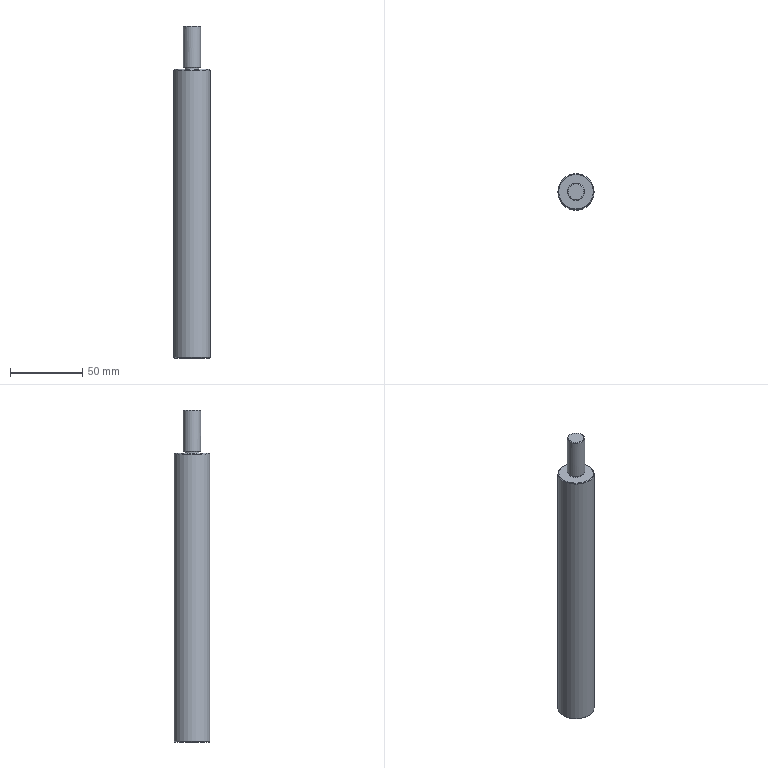Part | NX | features clamp shaft 2 | 1 solid | 13 faces | box 25 x 25 x 230 mm | volume 95439 mm3 | cone 5 | plane 4 | cylinder 4 | commonest cylinder face diameters 10 x1 12 x1 14 x1 25 x1
STEP:
#1=CARTESIAN_POINT('',(-5.5,0.,230.));
#2=VERTEX_POINT('',#1);
#3=CARTESIAN_POINT('',(0.,0.,230.));
#4=DIRECTION('',(0.,0.,-1.));
#5=DIRECTION('',(-1.,0.,0.));
#6=AXIS2_PLACEMENT_3D('',#3,#4,#5);
#7=CIRCLE('',#6,5.5);
#8=EDGE_CURVE('',#2,#2,#7,.T.);
#9=ORIENTED_EDGE('',*,*,#8,.F.);
#10=EDGE_LOOP('',(#9));
#11=FACE_BOUND('',#10,.T.);
#12=CARTESIAN_POINT('',(0.,0.,230.));
#13=DIRECTION('',(0.,0.,1.));
#14=DIRECTION('',(1.,0.,0.));
#15=AXIS2_PLACEMENT_3D('',#12,#13,#14);
#16=PLANE('',#15);
#17=ADVANCED_FACE('',(#11),#16,.T.);
#18=ORIENTED_EDGE('',*,*,#8,.T.);
#19=EDGE_LOOP('',(#18));
#20=FACE_BOUND('',#19,.T.);
#21=CARTESIAN_POINT('',(-6.,0.,229.5));
#22=VERTEX_POINT('',#21);
#23=CARTESIAN_POINT('',(0.,0.,229.5));
#24=DIRECTION('',(0.,0.,-1.));
#25=DIRECTION('',(-1.,0.,0.));
#26=AXIS2_PLACEMENT_3D('',#23,#24,#25);
#27=CIRCLE('',#26,6.);
#28=EDGE_CURVE('',#22,#22,#27,.T.);
#29=ORIENTED_EDGE('',*,*,#28,.F.);
#30=EDGE_LOOP('',(#29));
#31=FACE_BOUND('',#30,.T.);
#32=CARTESIAN_POINT('',(0.,0.,229.5));
#33=DIRECTION('',(0.,0.,-1.));
#34=DIRECTION('',(-1.,0.,0.));
#35=AXIS2_PLACEMENT_3D('',#32,#33,#34);
#36=CONICAL_SURFACE('',#35,6.,0.7854);
#37=ADVANCED_FACE('',(#20,#31),#36,.T.);
#38=ORIENTED_EDGE('',*,*,#28,.T.);
#39=EDGE_LOOP('',(#38));
#40=FACE_BOUND('',#39,.T.);
#41=CARTESIAN_POINT('',(6.,0.,201.5));
#42=VERTEX_POINT('',#41);
#43=CARTESIAN_POINT('',(0.,0.,201.5));
#44=DIRECTION('',(0.,0.,1.));
#45=DIRECTION('',(1.,0.,0.));
#46=AXIS2_PLACEMENT_3D('',#43,#44,#45);
#47=CIRCLE('',#46,6.);
#48=EDGE_CURVE('',#42,#42,#47,.F.);
#49=ORIENTED_EDGE('',*,*,#48,.F.);
#50=EDGE_LOOP('',(#49));
#51=FACE_BOUND('',#50,.T.);
#52=CARTESIAN_POINT('',(0.,0.,230.));
#53=DIRECTION('',(0.,0.,-1.));
#54=DIRECTION('',(-1.,0.,0.));
#55=AXIS2_PLACEMENT_3D('',#52,#53,#54);
#56=CYLINDRICAL_SURFACE('',#55,6.);
#57=ADVANCED_FACE('',(#40,#51),#56,.T.);
#58=CARTESIAN_POINT('',(0.,-5.5,201.));
#59=VERTEX_POINT('',#58);
#60=CARTESIAN_POINT('',(0.,0.,201.));
#61=DIRECTION('',(0.,0.,1.));
#62=DIRECTION('',(0.,-1.,0.));
#63=AXIS2_PLACEMENT_3D('',#60,#61,#62);
#64=CIRCLE('',#63,5.5);
#65=EDGE_CURVE('',#59,#59,#64,.T.);
#66=ORIENTED_EDGE('',*,*,#65,.T.);
#67=EDGE_LOOP('',(#66));
#68=FACE_BOUND('',#67,.T.);
#69=ORIENTED_EDGE('',*,*,#48,.T.);
#70=EDGE_LOOP('',(#69));
#71=FACE_BOUND('',#70,.T.);
#72=CARTESIAN_POINT('',(0.,0.,201.5));
#73=DIRECTION('',(0.,0.,1.));
#74=DIRECTION('',(0.,-1.,0.));
#75=AXIS2_PLACEMENT_3D('',#72,#73,#74);
#76=CONICAL_SURFACE('',#75,6.,0.7854);
#77=ADVANCED_FACE('',(#68,#71),#76,.T.);
#78=CARTESIAN_POINT('',(-5.,0.,201.));
#79=VERTEX_POINT('',#78);
#80=CARTESIAN_POINT('',(0.,0.,201.));
#81=DIRECTION('',(0.,0.,-1.));
#82=DIRECTION('',(-1.,0.,0.));
#83=AXIS2_PLACEMENT_3D('',#80,#81,#82);
#84=CIRCLE('',#83,5.);
#85=EDGE_CURVE('',#79,#79,#84,.T.);
#86=ORIENTED_EDGE('',*,*,#85,.F.);
#87=EDGE_LOOP('',(#86));
#88=FACE_BOUND('',#87,.T.);
#89=ORIENTED_EDGE('',*,*,#65,.F.);
#90=EDGE_LOOP('',(#89));
#91=FACE_BOUND('',#90,.T.);
#92=CARTESIAN_POINT('',(0.,0.,201.));
#93=DIRECTION('',(0.,0.,1.));
#94=DIRECTION('',(1.,0.,0.));
#95=AXIS2_PLACEMENT_3D('',#92,#93,#94);
#96=PLANE('',#95);
#97=ADVANCED_FACE('',(#88,#91),#96,.F.);
#98=CARTESIAN_POINT('',(0.,0.,42.206));
#99=VERTEX_POINT('',#98);
#100=VERTEX_LOOP('',#99);
#101=FACE_BOUND('',#100,.T.);
#102=CARTESIAN_POINT('',(-7.,0.,38.));
#103=VERTEX_POINT('',#102);
#104=CARTESIAN_POINT('',(0.,0.,38.));
#105=DIRECTION('',(0.,0.,-1.));
#106=DIRECTION('',(-1.,0.,0.));
#107=AXIS2_PLACEMENT_3D('',#104,#105,#106);
#108=CIRCLE('',#107,7.);
#109=EDGE_CURVE('',#103,#103,#108,.T.);
#110=ORIENTED_EDGE('',*,*,#109,.T.);
#111=EDGE_LOOP('',(#110));
#112=FACE_BOUND('',#111,.T.);
#113=CARTESIAN_POINT('',(0.,0.,38.));
#114=DIRECTION('',(0.,0.,-1.));
#115=DIRECTION('',(-1.,0.,0.));
#116=AXIS2_PLACEMENT_3D('',#113,#114,#115);
#117=CONICAL_SURFACE('',#116,7.,1.03);
#118=ADVANCED_FACE('',(#101,#112),#117,.F.);
#119=CARTESIAN_POINT('',(-5.,0.,200.));
#120=VERTEX_POINT('',#119);
#121=CARTESIAN_POINT('',(0.,0.,200.));
#122=DIRECTION('',(0.,0.,-1.));
#123=DIRECTION('',(-1.,0.,0.));
#124=AXIS2_PLACEMENT_3D('',#121,#122,#123);
#125=CIRCLE('',#124,5.);
#126=EDGE_CURVE('',#120,#120,#125,.T.);
#127=ORIENTED_EDGE('',*,*,#126,.F.);
#128=EDGE_LOOP('',(#127));
#129=FACE_BOUND('',#128,.T.);
#130=ORIENTED_EDGE('',*,*,#85,.T.);
#131=EDGE_LOOP('',(#130));
#132=FACE_BOUND('',#131,.T.);
#133=CARTESIAN_POINT('',(0.,0.,201.));
#134=DIRECTION('',(0.,0.,-1.));
#135=DIRECTION('',(-1.,0.,0.));
#136=AXIS2_PLACEMENT_3D('',#133,#134,#135);
#137=CYLINDRICAL_SURFACE('',#136,5.);
#138=ADVANCED_FACE('',(#129,#132),#137,.T.);
#139=ORIENTED_EDGE('',*,*,#109,.F.);
#140=EDGE_LOOP('',(#139));
#141=FACE_BOUND('',#140,.T.);
#142=CARTESIAN_POINT('',(-7.,0.,0.));
#143=VERTEX_POINT('',#142);
#144=CARTESIAN_POINT('',(0.,0.,0.));
#145=DIRECTION('',(0.,0.,-1.));
#146=DIRECTION('',(-1.,0.,0.));
#147=AXIS2_PLACEMENT_3D('',#144,#145,#146);
#148=CIRCLE('',#147,7.);
#149=EDGE_CURVE('',#143,#143,#148,.T.);
#150=ORIENTED_EDGE('',*,*,#149,.T.);
#151=EDGE_LOOP('',(#150));
#152=FACE_BOUND('',#151,.T.);
#153=CARTESIAN_POINT('',(0.,0.,0.));
#154=DIRECTION('',(0.,0.,-1.));
#155=DIRECTION('',(-1.,0.,0.));
#156=AXIS2_PLACEMENT_3D('',#153,#154,#155);
#157=CYLINDRICAL_SURFACE('',#156,7.);
#158=ADVANCED_FACE('',(#141,#152),#157,.F.);
#159=ORIENTED_EDGE('',*,*,#126,.T.);
#160=EDGE_LOOP('',(#159));
#161=FACE_BOUND('',#160,.T.);
#162=CARTESIAN_POINT('',(-12.,0.,200.));
#163=VERTEX_POINT('',#162);
#164=CARTESIAN_POINT('',(0.,0.,200.));
#165=DIRECTION('',(0.,0.,-1.));
#166=DIRECTION('',(-1.,0.,0.));
#167=AXIS2_PLACEMENT_3D('',#164,#165,#166);
#168=CIRCLE('',#167,12.);
#169=EDGE_CURVE('',#163,#163,#168,.T.);
#170=ORIENTED_EDGE('',*,*,#169,.F.);
#171=EDGE_LOOP('',(#170));
#172=FACE_BOUND('',#171,.T.);
#173=CARTESIAN_POINT('',(0.,0.,200.));
#174=DIRECTION('',(0.,0.,1.));
#175=DIRECTION('',(1.,0.,0.));
#176=AXIS2_PLACEMENT_3D('',#173,#174,#175);
#177=PLANE('',#176);
#178=ADVANCED_FACE('',(#161,#172),#177,.T.);
#179=CARTESIAN_POINT('',(12.,0.,0.));
#180=VERTEX_POINT('',#179);
#181=CARTESIAN_POINT('',(0.,0.,0.));
#182=DIRECTION('',(0.,0.,1.));
#183=DIRECTION('',(1.,0.,0.));
#184=AXIS2_PLACEMENT_3D('',#181,#182,#183);
#185=CIRCLE('',#184,12.);
#186=EDGE_CURVE('',#180,#180,#185,.T.);
#187=ORIENTED_EDGE('',*,*,#186,.F.);
#188=EDGE_LOOP('',(#187));
#189=FACE_BOUND('',#188,.T.);
#190=ORIENTED_EDGE('',*,*,#149,.F.);
#191=EDGE_LOOP('',(#190));
#192=FACE_BOUND('',#191,.T.);
#193=CARTESIAN_POINT('',(0.,0.,0.));
#194=DIRECTION('',(0.,0.,1.));
#195=DIRECTION('',(1.,0.,0.));
#196=AXIS2_PLACEMENT_3D('',#193,#194,#195);
#197=PLANE('',#196);
#198=ADVANCED_FACE('',(#189,#192),#197,.F.);
#199=CARTESIAN_POINT('',(-12.5,0.,199.5));
#200=VERTEX_POINT('',#199);
#201=CARTESIAN_POINT('',(0.,0.,199.5));
#202=DIRECTION('',(0.,0.,-1.));
#203=DIRECTION('',(-1.,0.,0.));
#204=AXIS2_PLACEMENT_3D('',#201,#202,#203);
#205=CIRCLE('',#204,12.5);
#206=EDGE_CURVE('',#200,#200,#205,.T.);
#207=ORIENTED_EDGE('',*,*,#206,.F.);
#208=EDGE_LOOP('',(#207));
#209=FACE_BOUND('',#208,.T.);
#210=ORIENTED_EDGE('',*,*,#169,.T.);
#211=EDGE_LOOP('',(#210));
#212=FACE_BOUND('',#211,.T.);
#213=CARTESIAN_POINT('',(0.,0.,199.5));
#214=DIRECTION('',(0.,0.,-1.));
#215=DIRECTION('',(-1.,0.,0.));
#216=AXIS2_PLACEMENT_3D('',#213,#214,#215);
#217=CONICAL_SURFACE('',#216,12.5,0.7854);
#218=ADVANCED_FACE('',(#209,#212),#217,.T.);
#219=CARTESIAN_POINT('',(-12.5,0.,0.5));
#220=VERTEX_POINT('',#219);
#221=CARTESIAN_POINT('',(0.,0.,0.5));
#222=DIRECTION('',(0.,0.,-1.));
#223=DIRECTION('',(-1.,0.,0.));
#224=AXIS2_PLACEMENT_3D('',#221,#222,#223);
#225=CIRCLE('',#224,12.5);
#226=EDGE_CURVE('',#220,#220,#225,.F.);
#227=ORIENTED_EDGE('',*,*,#226,.F.);
#228=EDGE_LOOP('',(#227));
#229=FACE_BOUND('',#228,.T.);
#230=ORIENTED_EDGE('',*,*,#186,.T.);
#231=EDGE_LOOP('',(#230));
#232=FACE_BOUND('',#231,.T.);
#233=CARTESIAN_POINT('',(0.,0.,0.5));
#234=DIRECTION('',(0.,0.,1.));
#235=DIRECTION('',(1.,0.,0.));
#236=AXIS2_PLACEMENT_3D('',#233,#234,#235);
#237=CONICAL_SURFACE('',#236,12.5,0.7854);
#238=ADVANCED_FACE('',(#229,#232),#237,.T.);
#239=ORIENTED_EDGE('',*,*,#226,.T.);
#240=EDGE_LOOP('',(#239));
#241=FACE_BOUND('',#240,.T.);
#242=ORIENTED_EDGE('',*,*,#206,.T.);
#243=EDGE_LOOP('',(#242));
#244=FACE_BOUND('',#243,.T.);
#245=CARTESIAN_POINT('',(0.,0.,200.));
#246=DIRECTION('',(0.,0.,-1.));
#247=DIRECTION('',(-1.,0.,0.));
#248=AXIS2_PLACEMENT_3D('',#245,#246,#247);
#249=CYLINDRICAL_SURFACE('',#248,12.5);
#250=ADVANCED_FACE('',(#241,#244),#249,.T.);
#251=CLOSED_SHELL('',(#17,#37,#57,#77,#97,#118,#138,#158,#178,#198,#218,#238,#250));
#252=MANIFOLD_SOLID_BREP('',#251);
#253=(LENGTH_UNIT()NAMED_UNIT(*)SI_UNIT(.MILLI.,.METRE.));
#254=UNCERTAINTY_MEASURE_WITH_UNIT(LENGTH_MEASURE(0.00001),#253,'','');
#255=(NAMED_UNIT(*)PLANE_ANGLE_UNIT()SI_UNIT($,.RADIAN.));
#256=(NAMED_UNIT(*)SI_UNIT($,.STERADIAN.)SOLID_ANGLE_UNIT());
#257=(GEOMETRIC_REPRESENTATION_CONTEXT(3)GLOBAL_UNCERTAINTY_ASSIGNED_CONTEXT((#254))GLOBAL_UNIT_ASSIGNED_CONTEXT((#253,#255,#256))REPRESENTATION_CONTEXT('',''));
#258=ADVANCED_BREP_SHAPE_REPRESENTATION('',(#252),#257);